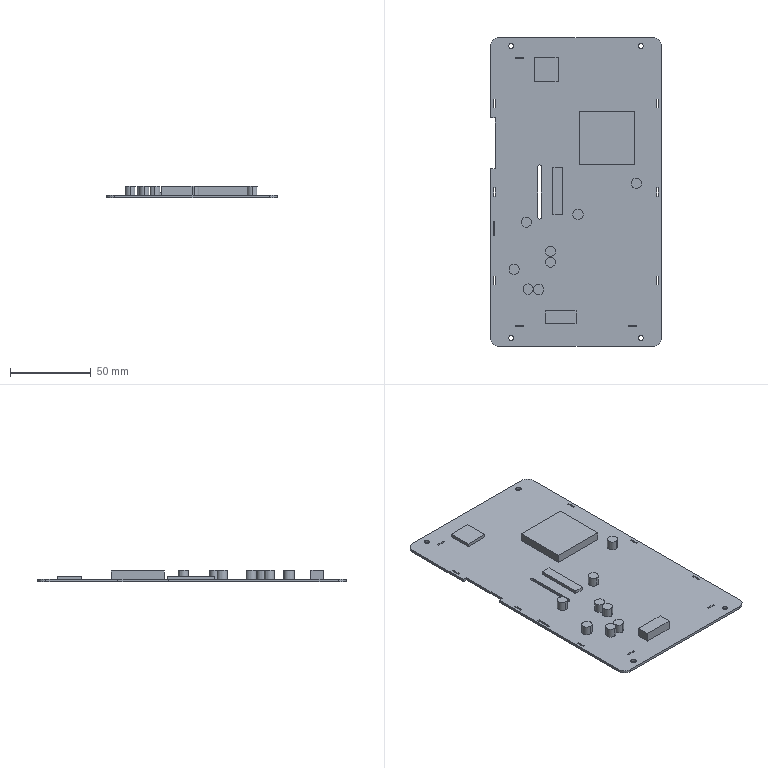Part | STEP file | DMG10600T070_01WTC_X2_8FEA658_3 | 1 solid | 110 faces | box 105.41 x 190.5 x 7.4 mm | volume 40629 mm3 | plane 80 | cylinder 30 | commonest cylinder face diameters 6.3 x16 3.2 x8 10.16 x4 2.032 x2